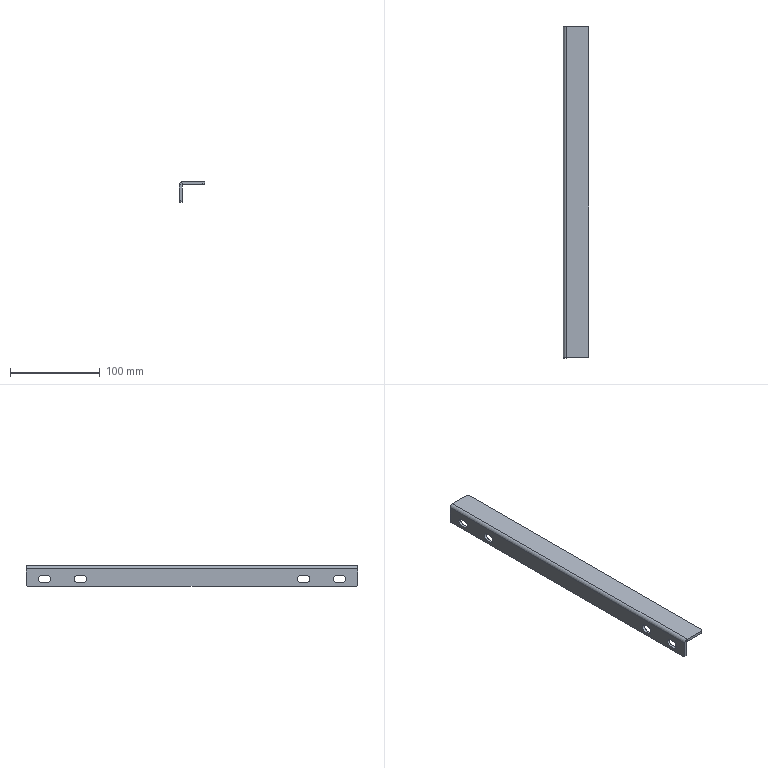Part | STEP file | Electrical cabinet support plate | 1 solid | 34 faces | box 28 x 370 x 23 mm | volume 51078 mm3 | plane 20 | cylinder 14 | commonest cylinder face diameters 8.5 x8 4 x4 1.2 x1 7.2 x1